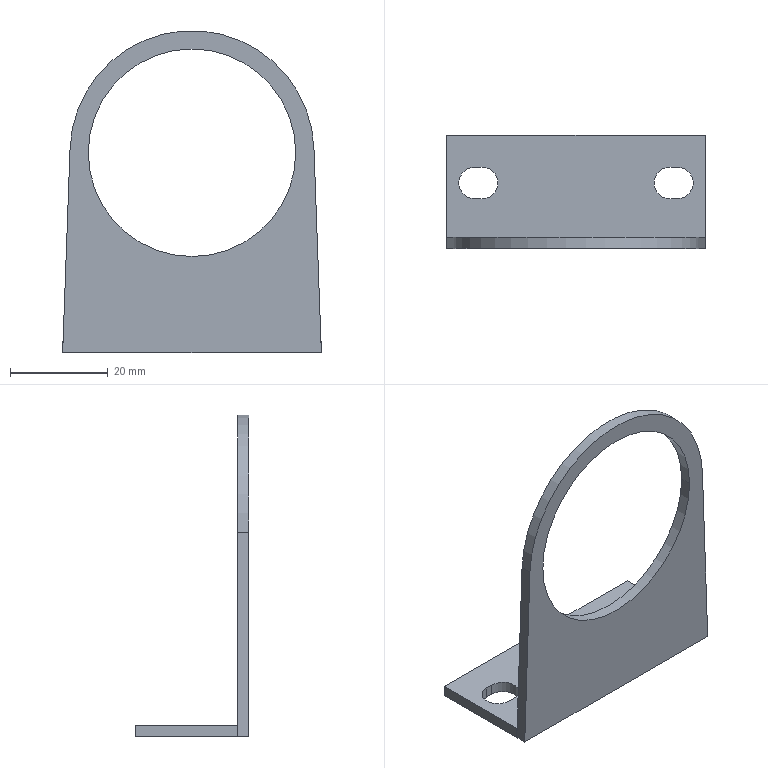Part | NX | 1 solid | 22 faces | box 53 x 23.3 x 66 mm | volume 6216 mm3 | plane 15 | cylinder 7 | commonest cylinder face diameters 6.5 x4 42.5 x2 50 x1
STEP:
#1=CARTESIAN_POINT('',(47.75,2.3,41.));
#2=VERTEX_POINT('',#1);
#3=CARTESIAN_POINT('',(5.25,2.3,41.));
#4=VERTEX_POINT('',#3);
#5=CARTESIAN_POINT('',(26.5,2.3,41.));
#6=DIRECTION('',(0.,1.,0.));
#7=DIRECTION('',(-1.,0.,0.));
#8=AXIS2_PLACEMENT_3D('',#5,#6,#7);
#9=CIRCLE('',#8,21.25);
#10=EDGE_CURVE('',#2,#4,#9,.T.);
#11=ORIENTED_EDGE('',*,*,#10,.T.);
#12=CARTESIAN_POINT('',(5.25,0.,41.));
#13=VERTEX_POINT('',#12);
#14=CARTESIAN_POINT('',(5.25,0.,41.));
#15=DIRECTION('',(0.,-1.,0.));
#16=VECTOR('',#15,1000.);
#17=LINE('',#14,#16);
#18=EDGE_CURVE('',#13,#4,#17,.F.);
#19=ORIENTED_EDGE('',*,*,#18,.F.);
#20=CARTESIAN_POINT('',(47.75,0.,41.));
#21=VERTEX_POINT('',#20);
#22=CARTESIAN_POINT('',(26.5,0.,41.));
#23=DIRECTION('',(0.,-1.,0.));
#24=DIRECTION('',(1.,0.,0.));
#25=AXIS2_PLACEMENT_3D('',#22,#23,#24);
#26=CIRCLE('',#25,21.25);
#27=EDGE_CURVE('',#13,#21,#26,.T.);
#28=ORIENTED_EDGE('',*,*,#27,.T.);
#29=CARTESIAN_POINT('',(47.75,0.,41.));
#30=DIRECTION('',(0.,-1.,0.));
#31=VECTOR('',#30,1000.);
#32=LINE('',#29,#31);
#33=EDGE_CURVE('',#21,#2,#32,.F.);
#34=ORIENTED_EDGE('',*,*,#33,.T.);
#35=EDGE_LOOP('',(#11,#19,#28,#34));
#36=FACE_BOUND('',#35,.T.);
#37=CARTESIAN_POINT('',(26.5,0.,41.));
#38=DIRECTION('',(0.,-1.,0.));
#39=DIRECTION('',(1.,0.,0.));
#40=AXIS2_PLACEMENT_3D('',#37,#38,#39);
#41=CYLINDRICAL_SURFACE('',#40,21.25);
#42=ADVANCED_FACE('',(#36),#41,.F.);
#43=CARTESIAN_POINT('',(45.75,16.75,2.3));
#44=VERTEX_POINT('',#43);
#45=CARTESIAN_POINT('',(45.75,10.25,2.3));
#46=VERTEX_POINT('',#45);
#47=CARTESIAN_POINT('',(45.75,13.5,2.3));
#48=DIRECTION('',(0.,0.,1.));
#49=DIRECTION('',(0.,1.,0.));
#50=AXIS2_PLACEMENT_3D('',#47,#48,#49);
#51=CIRCLE('',#50,3.25);
#52=EDGE_CURVE('',#44,#46,#51,.T.);
#53=ORIENTED_EDGE('',*,*,#52,.T.);
#54=CARTESIAN_POINT('',(45.75,10.25,0.));
#55=VERTEX_POINT('',#54);
#56=CARTESIAN_POINT('',(45.75,10.25,0.));
#57=DIRECTION('',(0.,0.,-1.));
#58=VECTOR('',#57,1000.);
#59=LINE('',#56,#58);
#60=EDGE_CURVE('',#46,#55,#59,.T.);
#61=ORIENTED_EDGE('',*,*,#60,.T.);
#62=CARTESIAN_POINT('',(45.75,16.75,0.));
#63=VERTEX_POINT('',#62);
#64=CARTESIAN_POINT('',(45.75,13.5,0.));
#65=DIRECTION('',(0.,0.,-1.));
#66=DIRECTION('',(0.,-1.,0.));
#67=AXIS2_PLACEMENT_3D('',#64,#65,#66);
#68=CIRCLE('',#67,3.25);
#69=EDGE_CURVE('',#55,#63,#68,.T.);
#70=ORIENTED_EDGE('',*,*,#69,.T.);
#71=CARTESIAN_POINT('',(45.75,16.75,0.));
#72=DIRECTION('',(0.,0.,-1.));
#73=VECTOR('',#72,1000.);
#74=LINE('',#71,#73);
#75=EDGE_CURVE('',#44,#63,#74,.T.);
#76=ORIENTED_EDGE('',*,*,#75,.F.);
#77=EDGE_LOOP('',(#53,#61,#70,#76));
#78=FACE_BOUND('',#77,.T.);
#79=CARTESIAN_POINT('',(45.75,13.5,0.));
#80=DIRECTION('',(0.,0.,-1.));
#81=DIRECTION('',(0.,1.,0.));
#82=AXIS2_PLACEMENT_3D('',#79,#80,#81);
#83=CYLINDRICAL_SURFACE('',#82,3.25);
#84=ADVANCED_FACE('',(#78),#83,.F.);
#85=CARTESIAN_POINT('',(0.,0.,0.));
#86=VERTEX_POINT('',#85);
#87=CARTESIAN_POINT('',(1.516,0.,41.904));
#88=VERTEX_POINT('',#87);
#89=CARTESIAN_POINT('',(0.,0.,0.));
#90=DIRECTION('',(0.03616,0.,0.9993));
#91=VECTOR('',#90,1000.);
#92=LINE('',#89,#91);
#93=EDGE_CURVE('',#86,#88,#92,.T.);
#94=ORIENTED_EDGE('',*,*,#93,.F.);
#95=CARTESIAN_POINT('',(53.,0.,0.));
#96=VERTEX_POINT('',#95);
#97=CARTESIAN_POINT('',(53.,0.,0.));
#98=DIRECTION('',(-1.,0.,0.));
#99=VECTOR('',#98,1000.);
#100=LINE('',#97,#99);
#101=EDGE_CURVE('',#96,#86,#100,.T.);
#102=ORIENTED_EDGE('',*,*,#101,.F.);
#103=CARTESIAN_POINT('',(51.484,0.,41.904));
#104=VERTEX_POINT('',#103);
#105=CARTESIAN_POINT('',(51.484,0.,41.904));
#106=DIRECTION('',(0.03616,0.,-0.9993));
#107=VECTOR('',#106,1000.);
#108=LINE('',#105,#107);
#109=EDGE_CURVE('',#104,#96,#108,.T.);
#110=ORIENTED_EDGE('',*,*,#109,.F.);
#111=CARTESIAN_POINT('',(26.5,0.,41.));
#112=DIRECTION('',(0.,1.,0.));
#113=DIRECTION('',(-0.9993,0.,0.03616));
#114=AXIS2_PLACEMENT_3D('',#111,#112,#113);
#115=CIRCLE('',#114,25.);
#116=EDGE_CURVE('',#88,#104,#115,.T.);
#117=ORIENTED_EDGE('',*,*,#116,.F.);
#118=EDGE_LOOP('',(#94,#102,#110,#117));
#119=FACE_BOUND('',#118,.T.);
#120=CARTESIAN_POINT('',(26.5,0.,41.));
#121=DIRECTION('',(0.,-1.,0.));
#122=DIRECTION('',(1.,0.,0.));
#123=AXIS2_PLACEMENT_3D('',#120,#121,#122);
#124=CIRCLE('',#123,21.25);
#125=EDGE_CURVE('',#21,#13,#124,.T.);
#126=ORIENTED_EDGE('',*,*,#125,.F.);
#127=ORIENTED_EDGE('',*,*,#27,.F.);
#128=EDGE_LOOP('',(#126,#127));
#129=FACE_BOUND('',#128,.T.);
#130=CARTESIAN_POINT('',(0.,0.,0.));
#131=DIRECTION('',(0.,1.,0.));
#132=DIRECTION('',(1.,0.,0.));
#133=AXIS2_PLACEMENT_3D('',#130,#131,#132);
#134=PLANE('',#133);
#135=ADVANCED_FACE('',(#119,#129),#134,.F.);
#136=CARTESIAN_POINT('',(1.516,2.3,41.904));
#137=VERTEX_POINT('',#136);
#138=CARTESIAN_POINT('',(0.08323,2.3,2.3));
#139=VERTEX_POINT('',#138);
#140=CARTESIAN_POINT('',(1.516,2.3,41.904));
#141=DIRECTION('',(-0.03616,0.,-0.9993));
#142=VECTOR('',#141,1000.);
#143=LINE('',#140,#142);
#144=EDGE_CURVE('',#137,#139,#143,.T.);
#145=ORIENTED_EDGE('',*,*,#144,.T.);
#146=CARTESIAN_POINT('',(0.,2.3,0.));
#147=VERTEX_POINT('',#146);
#148=CARTESIAN_POINT('',(0.08323,2.3,2.3));
#149=DIRECTION('',(-0.03616,0.,-0.9993));
#150=VECTOR('',#149,1000.);
#151=LINE('',#148,#150);
#152=EDGE_CURVE('',#139,#147,#151,.T.);
#153=ORIENTED_EDGE('',*,*,#152,.T.);
#154=CARTESIAN_POINT('',(0.,0.,0.));
#155=DIRECTION('',(0.,1.,0.));
#156=VECTOR('',#155,1000.);
#157=LINE('',#154,#156);
#158=EDGE_CURVE('',#86,#147,#157,.T.);
#159=ORIENTED_EDGE('',*,*,#158,.F.);
#160=ORIENTED_EDGE('',*,*,#93,.T.);
#161=CARTESIAN_POINT('',(1.516,0.,41.904));
#162=DIRECTION('',(0.,-1.,0.));
#163=VECTOR('',#162,1000.);
#164=LINE('',#161,#163);
#165=EDGE_CURVE('',#137,#88,#164,.T.);
#166=ORIENTED_EDGE('',*,*,#165,.F.);
#167=EDGE_LOOP('',(#145,#153,#159,#160,#166));
#168=FACE_BOUND('',#167,.T.);
#169=CARTESIAN_POINT('',(1.516,0.,41.904));
#170=DIRECTION('',(-0.9993,0.,0.03616));
#171=DIRECTION('',(0.,1.,0.));
#172=AXIS2_PLACEMENT_3D('',#169,#170,#171);
#173=PLANE('',#172);
#174=ADVANCED_FACE('',(#168),#173,.T.);
#175=CARTESIAN_POINT('',(52.917,2.3,2.3));
#176=VERTEX_POINT('',#175);
#177=CARTESIAN_POINT('',(52.917,2.3,2.3));
#178=DIRECTION('',(-1.,0.,0.));
#179=VECTOR('',#178,1000.);
#180=LINE('',#177,#179);
#181=EDGE_CURVE('',#176,#139,#180,.T.);
#182=ORIENTED_EDGE('',*,*,#181,.T.);
#183=ORIENTED_EDGE('',*,*,#144,.F.);
#184=CARTESIAN_POINT('',(51.484,2.3,41.904));
#185=VERTEX_POINT('',#184);
#186=CARTESIAN_POINT('',(26.5,2.3,41.));
#187=DIRECTION('',(0.,-1.,0.));
#188=DIRECTION('',(0.9993,0.,0.03616));
#189=AXIS2_PLACEMENT_3D('',#186,#187,#188);
#190=CIRCLE('',#189,25.);
#191=EDGE_CURVE('',#185,#137,#190,.T.);
#192=ORIENTED_EDGE('',*,*,#191,.F.);
#193=CARTESIAN_POINT('',(52.917,2.3,2.3));
#194=DIRECTION('',(-0.03616,0.,0.9993));
#195=VECTOR('',#194,1000.);
#196=LINE('',#193,#195);
#197=EDGE_CURVE('',#176,#185,#196,.T.);
#198=ORIENTED_EDGE('',*,*,#197,.F.);
#199=EDGE_LOOP('',(#182,#183,#192,#198));
#200=FACE_BOUND('',#199,.T.);
#201=ORIENTED_EDGE('',*,*,#10,.F.);
#202=CARTESIAN_POINT('',(26.5,2.3,41.));
#203=DIRECTION('',(0.,1.,0.));
#204=DIRECTION('',(-1.,0.,0.));
#205=AXIS2_PLACEMENT_3D('',#202,#203,#204);
#206=CIRCLE('',#205,21.25);
#207=EDGE_CURVE('',#4,#2,#206,.T.);
#208=ORIENTED_EDGE('',*,*,#207,.F.);
#209=EDGE_LOOP('',(#201,#208));
#210=FACE_BOUND('',#209,.T.);
#211=CARTESIAN_POINT('',(0.,2.3,0.));
#212=DIRECTION('',(0.,1.,0.));
#213=DIRECTION('',(1.,0.,0.));
#214=AXIS2_PLACEMENT_3D('',#211,#212,#213);
#215=PLANE('',#214);
#216=ADVANCED_FACE('',(#200,#210),#215,.T.);
#217=CARTESIAN_POINT('',(0.,2.3,2.3));
#218=VERTEX_POINT('',#217);
#219=CARTESIAN_POINT('',(0.,23.3,2.3));
#220=VERTEX_POINT('',#219);
#221=CARTESIAN_POINT('',(0.,2.3,2.3));
#222=DIRECTION('',(0.,1.,0.));
#223=VECTOR('',#222,1000.);
#224=LINE('',#221,#223);
#225=EDGE_CURVE('',#218,#220,#224,.T.);
#226=ORIENTED_EDGE('',*,*,#225,.F.);
#227=CARTESIAN_POINT('',(0.08323,2.3,2.3));
#228=DIRECTION('',(-1.,0.,0.));
#229=VECTOR('',#228,1000.);
#230=LINE('',#227,#229);
#231=EDGE_CURVE('',#139,#218,#230,.T.);
#232=ORIENTED_EDGE('',*,*,#231,.F.);
#233=ORIENTED_EDGE('',*,*,#181,.F.);
#234=CARTESIAN_POINT('',(53.,2.3,2.3));
#235=VERTEX_POINT('',#234);
#236=CARTESIAN_POINT('',(53.,2.3,2.3));
#237=DIRECTION('',(-1.,0.,0.));
#238=VECTOR('',#237,1000.);
#239=LINE('',#236,#238);
#240=EDGE_CURVE('',#235,#176,#239,.T.);
#241=ORIENTED_EDGE('',*,*,#240,.F.);
#242=CARTESIAN_POINT('',(53.,23.3,2.3));
#243=VERTEX_POINT('',#242);
#244=CARTESIAN_POINT('',(53.,23.3,2.3));
#245=DIRECTION('',(0.,-1.,0.));
#246=VECTOR('',#245,1000.);
#247=LINE('',#244,#246);
#248=EDGE_CURVE('',#243,#235,#247,.T.);
#249=ORIENTED_EDGE('',*,*,#248,.F.);
#250=CARTESIAN_POINT('',(0.,23.3,2.3));
#251=DIRECTION('',(1.,0.,0.));
#252=VECTOR('',#251,1000.);
#253=LINE('',#250,#252);
#254=EDGE_CURVE('',#220,#243,#253,.T.);
#255=ORIENTED_EDGE('',*,*,#254,.F.);
#256=EDGE_LOOP('',(#226,#232,#233,#241,#249,#255));
#257=FACE_BOUND('',#256,.T.);
#258=ORIENTED_EDGE('',*,*,#52,.F.);
#259=CARTESIAN_POINT('',(47.25,16.75,2.3));
#260=VERTEX_POINT('',#259);
#261=CARTESIAN_POINT('',(47.25,16.75,2.3));
#262=DIRECTION('',(-1.,0.,0.));
#263=VECTOR('',#262,1000.);
#264=LINE('',#261,#263);
#265=EDGE_CURVE('',#260,#44,#264,.T.);
#266=ORIENTED_EDGE('',*,*,#265,.F.);
#267=CARTESIAN_POINT('',(47.25,10.25,2.3));
#268=VERTEX_POINT('',#267);
#269=CARTESIAN_POINT('',(47.25,13.5,2.3));
#270=DIRECTION('',(0.,0.,1.));
#271=DIRECTION('',(0.,-1.,0.));
#272=AXIS2_PLACEMENT_3D('',#269,#270,#271);
#273=CIRCLE('',#272,3.25);
#274=EDGE_CURVE('',#268,#260,#273,.T.);
#275=ORIENTED_EDGE('',*,*,#274,.F.);
#276=CARTESIAN_POINT('',(45.75,10.25,2.3));
#277=DIRECTION('',(1.,0.,0.));
#278=VECTOR('',#277,1000.);
#279=LINE('',#276,#278);
#280=EDGE_CURVE('',#46,#268,#279,.T.);
#281=ORIENTED_EDGE('',*,*,#280,.F.);
#282=EDGE_LOOP('',(#258,#266,#275,#281));
#283=FACE_BOUND('',#282,.T.);
#284=CARTESIAN_POINT('',(5.75,16.75,2.3));
#285=VERTEX_POINT('',#284);
#286=CARTESIAN_POINT('',(5.75,10.25,2.3));
#287=VERTEX_POINT('',#286);
#288=CARTESIAN_POINT('',(5.75,13.5,2.3));
#289=DIRECTION('',(0.,0.,1.));
#290=DIRECTION('',(0.,1.,0.));
#291=AXIS2_PLACEMENT_3D('',#288,#289,#290);
#292=CIRCLE('',#291,3.25);
#293=EDGE_CURVE('',#285,#287,#292,.T.);
#294=ORIENTED_EDGE('',*,*,#293,.F.);
#295=CARTESIAN_POINT('',(7.25,16.75,2.3));
#296=VERTEX_POINT('',#295);
#297=CARTESIAN_POINT('',(7.25,16.75,2.3));
#298=DIRECTION('',(-1.,0.,0.));
#299=VECTOR('',#298,1000.);
#300=LINE('',#297,#299);
#301=EDGE_CURVE('',#296,#285,#300,.T.);
#302=ORIENTED_EDGE('',*,*,#301,.F.);
#303=CARTESIAN_POINT('',(7.25,10.25,2.3));
#304=VERTEX_POINT('',#303);
#305=CARTESIAN_POINT('',(7.25,13.5,2.3));
#306=DIRECTION('',(0.,0.,1.));
#307=DIRECTION('',(0.,-1.,0.));
#308=AXIS2_PLACEMENT_3D('',#305,#306,#307);
#309=CIRCLE('',#308,3.25);
#310=EDGE_CURVE('',#304,#296,#309,.T.);
#311=ORIENTED_EDGE('',*,*,#310,.F.);
#312=CARTESIAN_POINT('',(5.75,10.25,2.3));
#313=DIRECTION('',(1.,0.,0.));
#314=VECTOR('',#313,1000.);
#315=LINE('',#312,#314);
#316=EDGE_CURVE('',#287,#304,#315,.T.);
#317=ORIENTED_EDGE('',*,*,#316,.F.);
#318=EDGE_LOOP('',(#294,#302,#311,#317));
#319=FACE_BOUND('',#318,.T.);
#320=CARTESIAN_POINT('',(0.,0.,2.3));
#321=DIRECTION('',(0.,0.,1.));
#322=DIRECTION('',(1.,0.,0.));
#323=AXIS2_PLACEMENT_3D('',#320,#321,#322);
#324=PLANE('',#323);
#325=ADVANCED_FACE('',(#257,#283,#319),#324,.T.);
#326=ORIENTED_EDGE('',*,*,#225,.T.);
#327=CARTESIAN_POINT('',(0.,23.3,0.));
#328=VERTEX_POINT('',#327);
#329=CARTESIAN_POINT('',(0.,23.3,0.));
#330=DIRECTION('',(0.,0.,1.));
#331=VECTOR('',#330,1000.);
#332=LINE('',#329,#331);
#333=EDGE_CURVE('',#328,#220,#332,.T.);
#334=ORIENTED_EDGE('',*,*,#333,.F.);
#335=CARTESIAN_POINT('',(0.,23.3,0.));
#336=DIRECTION('',(0.,-1.,0.));
#337=VECTOR('',#336,1000.);
#338=LINE('',#335,#337);
#339=EDGE_CURVE('',#328,#147,#338,.T.);
#340=ORIENTED_EDGE('',*,*,#339,.T.);
#341=CARTESIAN_POINT('',(0.,2.3,0.));
#342=DIRECTION('',(0.,0.,1.));
#343=VECTOR('',#342,1000.);
#344=LINE('',#341,#343);
#345=EDGE_CURVE('',#147,#218,#344,.T.);
#346=ORIENTED_EDGE('',*,*,#345,.T.);
#347=EDGE_LOOP('',(#326,#334,#340,#346));
#348=FACE_BOUND('',#347,.T.);
#349=CARTESIAN_POINT('',(0.,2.3,0.));
#350=DIRECTION('',(-1.,0.,0.));
#351=DIRECTION('',(0.,0.,1.));
#352=AXIS2_PLACEMENT_3D('',#349,#350,#351);
#353=PLANE('',#352);
#354=ADVANCED_FACE('',(#348),#353,.T.);
#355=ORIENTED_EDGE('',*,*,#152,.F.);
#356=ORIENTED_EDGE('',*,*,#231,.T.);
#357=ORIENTED_EDGE('',*,*,#345,.F.);
#358=EDGE_LOOP('',(#355,#356,#357));
#359=FACE_BOUND('',#358,.T.);
#360=CARTESIAN_POINT('',(53.,2.3,0.));
#361=DIRECTION('',(0.,-1.,0.));
#362=DIRECTION('',(0.,0.,-1.));
#363=AXIS2_PLACEMENT_3D('',#360,#361,#362);
#364=PLANE('',#363);
#365=ADVANCED_FACE('',(#359),#364,.T.);
#366=CARTESIAN_POINT('',(53.,2.3,0.));
#367=VERTEX_POINT('',#366);
#368=CARTESIAN_POINT('',(53.,0.,0.));
#369=DIRECTION('',(0.,1.,0.));
#370=VECTOR('',#369,1000.);
#371=LINE('',#368,#370);
#372=EDGE_CURVE('',#96,#367,#371,.T.);
#373=ORIENTED_EDGE('',*,*,#372,.F.);
#374=ORIENTED_EDGE('',*,*,#101,.T.);
#375=ORIENTED_EDGE('',*,*,#158,.T.);
#376=ORIENTED_EDGE('',*,*,#339,.F.);
#377=CARTESIAN_POINT('',(53.,23.3,0.));
#378=VERTEX_POINT('',#377);
#379=CARTESIAN_POINT('',(53.,23.3,0.));
#380=DIRECTION('',(-1.,0.,0.));
#381=VECTOR('',#380,1000.);
#382=LINE('',#379,#381);
#383=EDGE_CURVE('',#378,#328,#382,.T.);
#384=ORIENTED_EDGE('',*,*,#383,.F.);
#385=CARTESIAN_POINT('',(53.,2.3,0.));
#386=DIRECTION('',(0.,1.,0.));
#387=VECTOR('',#386,1000.);
#388=LINE('',#385,#387);
#389=EDGE_CURVE('',#367,#378,#388,.T.);
#390=ORIENTED_EDGE('',*,*,#389,.F.);
#391=EDGE_LOOP('',(#373,#374,#375,#376,#384,#390));
#392=FACE_BOUND('',#391,.T.);
#393=CARTESIAN_POINT('',(7.25,16.75,0.));
#394=VERTEX_POINT('',#393);
#395=CARTESIAN_POINT('',(5.75,16.75,0.));
#396=VERTEX_POINT('',#395);
#397=CARTESIAN_POINT('',(7.25,16.75,0.));
#398=DIRECTION('',(-1.,0.,0.));
#399=VECTOR('',#398,1000.);
#400=LINE('',#397,#399);
#401=EDGE_CURVE('',#394,#396,#400,.T.);
#402=ORIENTED_EDGE('',*,*,#401,.T.);
#403=CARTESIAN_POINT('',(5.75,10.25,0.));
#404=VERTEX_POINT('',#403);
#405=CARTESIAN_POINT('',(5.75,13.5,0.));
#406=DIRECTION('',(0.,0.,-1.));
#407=DIRECTION('',(0.,-1.,0.));
#408=AXIS2_PLACEMENT_3D('',#405,#406,#407);
#409=CIRCLE('',#408,3.25);
#410=EDGE_CURVE('',#404,#396,#409,.T.);
#411=ORIENTED_EDGE('',*,*,#410,.F.);
#412=CARTESIAN_POINT('',(7.25,10.25,0.));
#413=VERTEX_POINT('',#412);
#414=CARTESIAN_POINT('',(5.75,10.25,0.));
#415=DIRECTION('',(1.,0.,0.));
#416=VECTOR('',#415,1000.);
#417=LINE('',#414,#416);
#418=EDGE_CURVE('',#404,#413,#417,.T.);
#419=ORIENTED_EDGE('',*,*,#418,.T.);
#420=CARTESIAN_POINT('',(7.25,13.5,0.));
#421=DIRECTION('',(0.,0.,-1.));
#422=DIRECTION('',(0.,1.,0.));
#423=AXIS2_PLACEMENT_3D('',#420,#421,#422);
#424=CIRCLE('',#423,3.25);
#425=EDGE_CURVE('',#394,#413,#424,.T.);
#426=ORIENTED_EDGE('',*,*,#425,.F.);
#427=EDGE_LOOP('',(#402,#411,#419,#426));
#428=FACE_BOUND('',#427,.T.);
#429=CARTESIAN_POINT('',(47.25,16.75,0.));
#430=VERTEX_POINT('',#429);
#431=CARTESIAN_POINT('',(47.25,16.75,0.));
#432=DIRECTION('',(-1.,0.,0.));
#433=VECTOR('',#432,1000.);
#434=LINE('',#431,#433);
#435=EDGE_CURVE('',#430,#63,#434,.T.);
#436=ORIENTED_EDGE('',*,*,#435,.T.);
#437=ORIENTED_EDGE('',*,*,#69,.F.);
#438=CARTESIAN_POINT('',(47.25,10.25,0.));
#439=VERTEX_POINT('',#438);
#440=CARTESIAN_POINT('',(45.75,10.25,0.));
#441=DIRECTION('',(1.,0.,0.));
#442=VECTOR('',#441,1000.);
#443=LINE('',#440,#442);
#444=EDGE_CURVE('',#55,#439,#443,.T.);
#445=ORIENTED_EDGE('',*,*,#444,.T.);
#446=CARTESIAN_POINT('',(47.25,13.5,0.));
#447=DIRECTION('',(0.,0.,-1.));
#448=DIRECTION('',(0.,1.,0.));
#449=AXIS2_PLACEMENT_3D('',#446,#447,#448);
#450=CIRCLE('',#449,3.25);
#451=EDGE_CURVE('',#430,#439,#450,.T.);
#452=ORIENTED_EDGE('',*,*,#451,.F.);
#453=EDGE_LOOP('',(#436,#437,#445,#452));
#454=FACE_BOUND('',#453,.T.);
#455=CARTESIAN_POINT('',(0.,0.,0.));
#456=DIRECTION('',(0.,0.,-1.));
#457=DIRECTION('',(0.,-1.,0.));
#458=AXIS2_PLACEMENT_3D('',#455,#456,#457);
#459=PLANE('',#458);
#460=ADVANCED_FACE('',(#392,#428,#454),#459,.T.);
#461=CARTESIAN_POINT('',(53.,2.3,0.));
#462=DIRECTION('',(-0.03616,0.,0.9993));
#463=VECTOR('',#462,1000.);
#464=LINE('',#461,#463);
#465=EDGE_CURVE('',#367,#176,#464,.T.);
#466=ORIENTED_EDGE('',*,*,#465,.T.);
#467=ORIENTED_EDGE('',*,*,#197,.T.);
#468=CARTESIAN_POINT('',(51.484,2.3,41.904));
#469=DIRECTION('',(0.,-1.,0.));
#470=VECTOR('',#469,1000.);
#471=LINE('',#468,#470);
#472=EDGE_CURVE('',#185,#104,#471,.T.);
#473=ORIENTED_EDGE('',*,*,#472,.T.);
#474=ORIENTED_EDGE('',*,*,#109,.T.);
#475=ORIENTED_EDGE('',*,*,#372,.T.);
#476=EDGE_LOOP('',(#466,#467,#473,#474,#475));
#477=FACE_BOUND('',#476,.T.);
#478=CARTESIAN_POINT('',(53.,0.,0.));
#479=DIRECTION('',(0.9993,0.,0.03616));
#480=DIRECTION('',(0.,-1.,0.));
#481=AXIS2_PLACEMENT_3D('',#478,#479,#480);
#482=PLANE('',#481);
#483=ADVANCED_FACE('',(#477),#482,.T.);
#484=ORIENTED_EDGE('',*,*,#465,.F.);
#485=CARTESIAN_POINT('',(53.,2.3,0.));
#486=DIRECTION('',(0.,0.,1.));
#487=VECTOR('',#486,1000.);
#488=LINE('',#485,#487);
#489=EDGE_CURVE('',#367,#235,#488,.T.);
#490=ORIENTED_EDGE('',*,*,#489,.T.);
#491=ORIENTED_EDGE('',*,*,#240,.T.);
#492=EDGE_LOOP('',(#484,#490,#491));
#493=FACE_BOUND('',#492,.T.);
#494=CARTESIAN_POINT('',(53.,2.3,0.));
#495=DIRECTION('',(0.,-1.,0.));
#496=DIRECTION('',(0.,0.,-1.));
#497=AXIS2_PLACEMENT_3D('',#494,#495,#496);
#498=PLANE('',#497);
#499=ADVANCED_FACE('',(#493),#498,.T.);
#500=ORIENTED_EDGE('',*,*,#248,.T.);
#501=ORIENTED_EDGE('',*,*,#489,.F.);
#502=ORIENTED_EDGE('',*,*,#389,.T.);
#503=CARTESIAN_POINT('',(53.,23.3,0.));
#504=DIRECTION('',(0.,0.,1.));
#505=VECTOR('',#504,1000.);
#506=LINE('',#503,#505);
#507=EDGE_CURVE('',#378,#243,#506,.T.);
#508=ORIENTED_EDGE('',*,*,#507,.T.);
#509=EDGE_LOOP('',(#500,#501,#502,#508));
#510=FACE_BOUND('',#509,.T.);
#511=CARTESIAN_POINT('',(53.,23.3,0.));
#512=DIRECTION('',(1.,0.,0.));
#513=DIRECTION('',(0.,1.,0.));
#514=AXIS2_PLACEMENT_3D('',#511,#512,#513);
#515=PLANE('',#514);
#516=ADVANCED_FACE('',(#510),#515,.T.);
#517=ORIENTED_EDGE('',*,*,#254,.T.);
#518=ORIENTED_EDGE('',*,*,#507,.F.);
#519=ORIENTED_EDGE('',*,*,#383,.T.);
#520=ORIENTED_EDGE('',*,*,#333,.T.);
#521=EDGE_LOOP('',(#517,#518,#519,#520));
#522=FACE_BOUND('',#521,.T.);
#523=CARTESIAN_POINT('',(0.,23.3,0.));
#524=DIRECTION('',(0.,1.,0.));
#525=DIRECTION('',(1.,0.,0.));
#526=AXIS2_PLACEMENT_3D('',#523,#524,#525);
#527=PLANE('',#526);
#528=ADVANCED_FACE('',(#522),#527,.T.);
#529=ORIENTED_EDGE('',*,*,#191,.T.);
#530=ORIENTED_EDGE('',*,*,#165,.T.);
#531=ORIENTED_EDGE('',*,*,#116,.T.);
#532=ORIENTED_EDGE('',*,*,#472,.F.);
#533=EDGE_LOOP('',(#529,#530,#531,#532));
#534=FACE_BOUND('',#533,.T.);
#535=CARTESIAN_POINT('',(26.5,0.,41.));
#536=DIRECTION('',(0.,-1.,0.));
#537=DIRECTION('',(-0.9993,0.,0.03616));
#538=AXIS2_PLACEMENT_3D('',#535,#536,#537);
#539=CYLINDRICAL_SURFACE('',#538,25.);
#540=ADVANCED_FACE('',(#534),#539,.T.);
#541=ORIENTED_EDGE('',*,*,#301,.T.);
#542=CARTESIAN_POINT('',(5.75,16.75,0.));
#543=DIRECTION('',(0.,0.,-1.));
#544=VECTOR('',#543,1000.);
#545=LINE('',#542,#544);
#546=EDGE_CURVE('',#285,#396,#545,.T.);
#547=ORIENTED_EDGE('',*,*,#546,.T.);
#548=ORIENTED_EDGE('',*,*,#401,.F.);
#549=CARTESIAN_POINT('',(7.25,16.75,0.));
#550=DIRECTION('',(0.,0.,-1.));
#551=VECTOR('',#550,1000.);
#552=LINE('',#549,#551);
#553=EDGE_CURVE('',#296,#394,#552,.T.);
#554=ORIENTED_EDGE('',*,*,#553,.F.);
#555=EDGE_LOOP('',(#541,#547,#548,#554));
#556=FACE_BOUND('',#555,.T.);
#557=CARTESIAN_POINT('',(7.25,16.75,0.));
#558=DIRECTION('',(0.,-1.,0.));
#559=DIRECTION('',(0.,0.,-1.));
#560=AXIS2_PLACEMENT_3D('',#557,#558,#559);
#561=PLANE('',#560);
#562=ADVANCED_FACE('',(#556),#561,.T.);
#563=ORIENTED_EDGE('',*,*,#310,.T.);
#564=ORIENTED_EDGE('',*,*,#553,.T.);
#565=ORIENTED_EDGE('',*,*,#425,.T.);
#566=CARTESIAN_POINT('',(7.25,10.25,0.));
#567=DIRECTION('',(0.,0.,-1.));
#568=VECTOR('',#567,1000.);
#569=LINE('',#566,#568);
#570=EDGE_CURVE('',#304,#413,#569,.T.);
#571=ORIENTED_EDGE('',*,*,#570,.F.);
#572=EDGE_LOOP('',(#563,#564,#565,#571));
#573=FACE_BOUND('',#572,.T.);
#574=CARTESIAN_POINT('',(7.25,13.5,0.));
#575=DIRECTION('',(0.,0.,-1.));
#576=DIRECTION('',(0.,-1.,0.));
#577=AXIS2_PLACEMENT_3D('',#574,#575,#576);
#578=CYLINDRICAL_SURFACE('',#577,3.25);
#579=ADVANCED_FACE('',(#573),#578,.F.);
#580=ORIENTED_EDGE('',*,*,#316,.T.);
#581=ORIENTED_EDGE('',*,*,#570,.T.);
#582=ORIENTED_EDGE('',*,*,#418,.F.);
#583=CARTESIAN_POINT('',(5.75,10.25,0.));
#584=DIRECTION('',(0.,0.,-1.));
#585=VECTOR('',#584,1000.);
#586=LINE('',#583,#585);
#587=EDGE_CURVE('',#287,#404,#586,.T.);
#588=ORIENTED_EDGE('',*,*,#587,.F.);
#589=EDGE_LOOP('',(#580,#581,#582,#588));
#590=FACE_BOUND('',#589,.T.);
#591=CARTESIAN_POINT('',(5.75,10.25,0.));
#592=DIRECTION('',(0.,1.,0.));
#593=DIRECTION('',(1.,0.,0.));
#594=AXIS2_PLACEMENT_3D('',#591,#592,#593);
#595=PLANE('',#594);
#596=ADVANCED_FACE('',(#590),#595,.T.);
#597=ORIENTED_EDGE('',*,*,#293,.T.);
#598=ORIENTED_EDGE('',*,*,#587,.T.);
#599=ORIENTED_EDGE('',*,*,#410,.T.);
#600=ORIENTED_EDGE('',*,*,#546,.F.);
#601=EDGE_LOOP('',(#597,#598,#599,#600));
#602=FACE_BOUND('',#601,.T.);
#603=CARTESIAN_POINT('',(5.75,13.5,0.));
#604=DIRECTION('',(0.,0.,-1.));
#605=DIRECTION('',(0.,1.,0.));
#606=AXIS2_PLACEMENT_3D('',#603,#604,#605);
#607=CYLINDRICAL_SURFACE('',#606,3.25);
#608=ADVANCED_FACE('',(#602),#607,.F.);
#609=ORIENTED_EDGE('',*,*,#265,.T.);
#610=ORIENTED_EDGE('',*,*,#75,.T.);
#611=ORIENTED_EDGE('',*,*,#435,.F.);
#612=CARTESIAN_POINT('',(47.25,16.75,0.));
#613=DIRECTION('',(0.,0.,-1.));
#614=VECTOR('',#613,1000.);
#615=LINE('',#612,#614);
#616=EDGE_CURVE('',#260,#430,#615,.T.);
#617=ORIENTED_EDGE('',*,*,#616,.F.);
#618=EDGE_LOOP('',(#609,#610,#611,#617));
#619=FACE_BOUND('',#618,.T.);
#620=CARTESIAN_POINT('',(47.25,16.75,0.));
#621=DIRECTION('',(0.,-1.,0.));
#622=DIRECTION('',(0.,0.,-1.));
#623=AXIS2_PLACEMENT_3D('',#620,#621,#622);
#624=PLANE('',#623);
#625=ADVANCED_FACE('',(#619),#624,.T.);
#626=ORIENTED_EDGE('',*,*,#274,.T.);
#627=ORIENTED_EDGE('',*,*,#616,.T.);
#628=ORIENTED_EDGE('',*,*,#451,.T.);
#629=CARTESIAN_POINT('',(47.25,10.25,0.));
#630=DIRECTION('',(0.,0.,-1.));
#631=VECTOR('',#630,1000.);
#632=LINE('',#629,#631);
#633=EDGE_CURVE('',#268,#439,#632,.T.);
#634=ORIENTED_EDGE('',*,*,#633,.F.);
#635=EDGE_LOOP('',(#626,#627,#628,#634));
#636=FACE_BOUND('',#635,.T.);
#637=CARTESIAN_POINT('',(47.25,13.5,0.));
#638=DIRECTION('',(0.,0.,-1.));
#639=DIRECTION('',(0.,-1.,0.));
#640=AXIS2_PLACEMENT_3D('',#637,#638,#639);
#641=CYLINDRICAL_SURFACE('',#640,3.25);
#642=ADVANCED_FACE('',(#636),#641,.F.);
#643=ORIENTED_EDGE('',*,*,#280,.T.);
#644=ORIENTED_EDGE('',*,*,#633,.T.);
#645=ORIENTED_EDGE('',*,*,#444,.F.);
#646=ORIENTED_EDGE('',*,*,#60,.F.);
#647=EDGE_LOOP('',(#643,#644,#645,#646));
#648=FACE_BOUND('',#647,.T.);
#649=CARTESIAN_POINT('',(45.75,10.25,0.));
#650=DIRECTION('',(0.,1.,0.));
#651=DIRECTION('',(1.,0.,0.));
#652=AXIS2_PLACEMENT_3D('',#649,#650,#651);
#653=PLANE('',#652);
#654=ADVANCED_FACE('',(#648),#653,.T.);
#655=ORIENTED_EDGE('',*,*,#125,.T.);
#656=ORIENTED_EDGE('',*,*,#18,.T.);
#657=ORIENTED_EDGE('',*,*,#207,.T.);
#658=ORIENTED_EDGE('',*,*,#33,.F.);
#659=EDGE_LOOP('',(#655,#656,#657,#658));
#660=FACE_BOUND('',#659,.T.);
#661=CARTESIAN_POINT('',(26.5,0.,41.));
#662=DIRECTION('',(0.,-1.,0.));
#663=DIRECTION('',(1.,0.,0.));
#664=AXIS2_PLACEMENT_3D('',#661,#662,#663);
#665=CYLINDRICAL_SURFACE('',#664,21.25);
#666=ADVANCED_FACE('',(#660),#665,.F.);
#667=CLOSED_SHELL('',(#42,#84,#135,#174,#216,#325,#354,#365,#460,#483,#499,#516,#528,#540,#562,#579,#596,#608,#625,#642,#654,#666));
#668=MANIFOLD_SOLID_BREP('',#667);
#669=(LENGTH_UNIT()NAMED_UNIT(*)SI_UNIT(.MILLI.,.METRE.));
#670=UNCERTAINTY_MEASURE_WITH_UNIT(LENGTH_MEASURE(0.00001),#669,'','');
#671=(NAMED_UNIT(*)PLANE_ANGLE_UNIT()SI_UNIT($,.RADIAN.));
#672=(NAMED_UNIT(*)SI_UNIT($,.STERADIAN.)SOLID_ANGLE_UNIT());
#673=(GEOMETRIC_REPRESENTATION_CONTEXT(3)GLOBAL_UNCERTAINTY_ASSIGNED_CONTEXT((#670))GLOBAL_UNIT_ASSIGNED_CONTEXT((#669,#671,#672))REPRESENTATION_CONTEXT('',''));
#674=ADVANCED_BREP_SHAPE_REPRESENTATION('',(#668),#673);